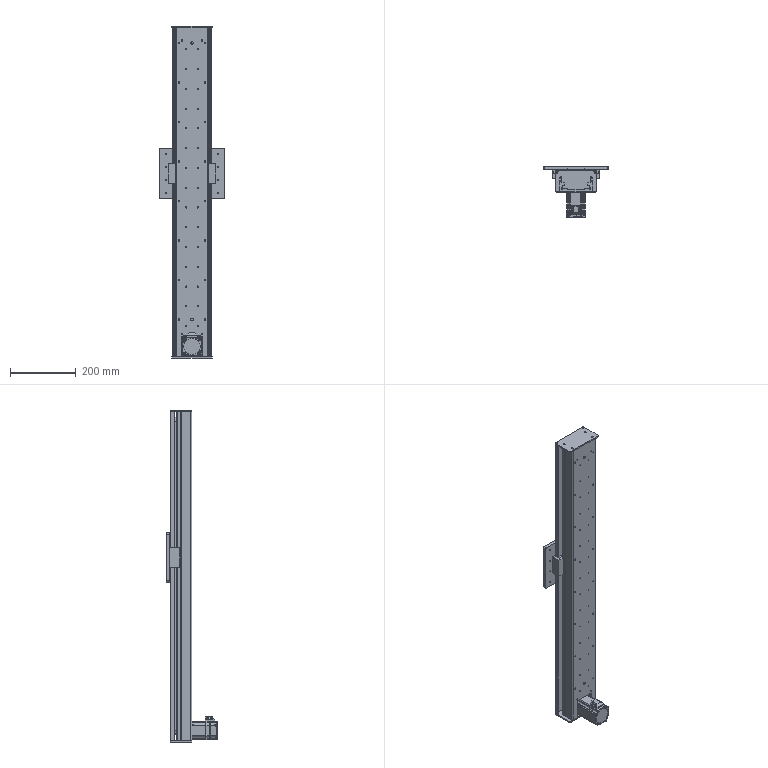Part | SolidWorks | features InContextFeatHolder 1, LocalLPattern 1 | 36 solids | 3251 faces | volume 2926027 mm3 | cone 1371 | cylinder 1050 | plane 743 | spline 87 | commonest cylinder face diameters 3.3 x176 4.5 x148 6 x83 1 x72 3.2 x57 8 x50